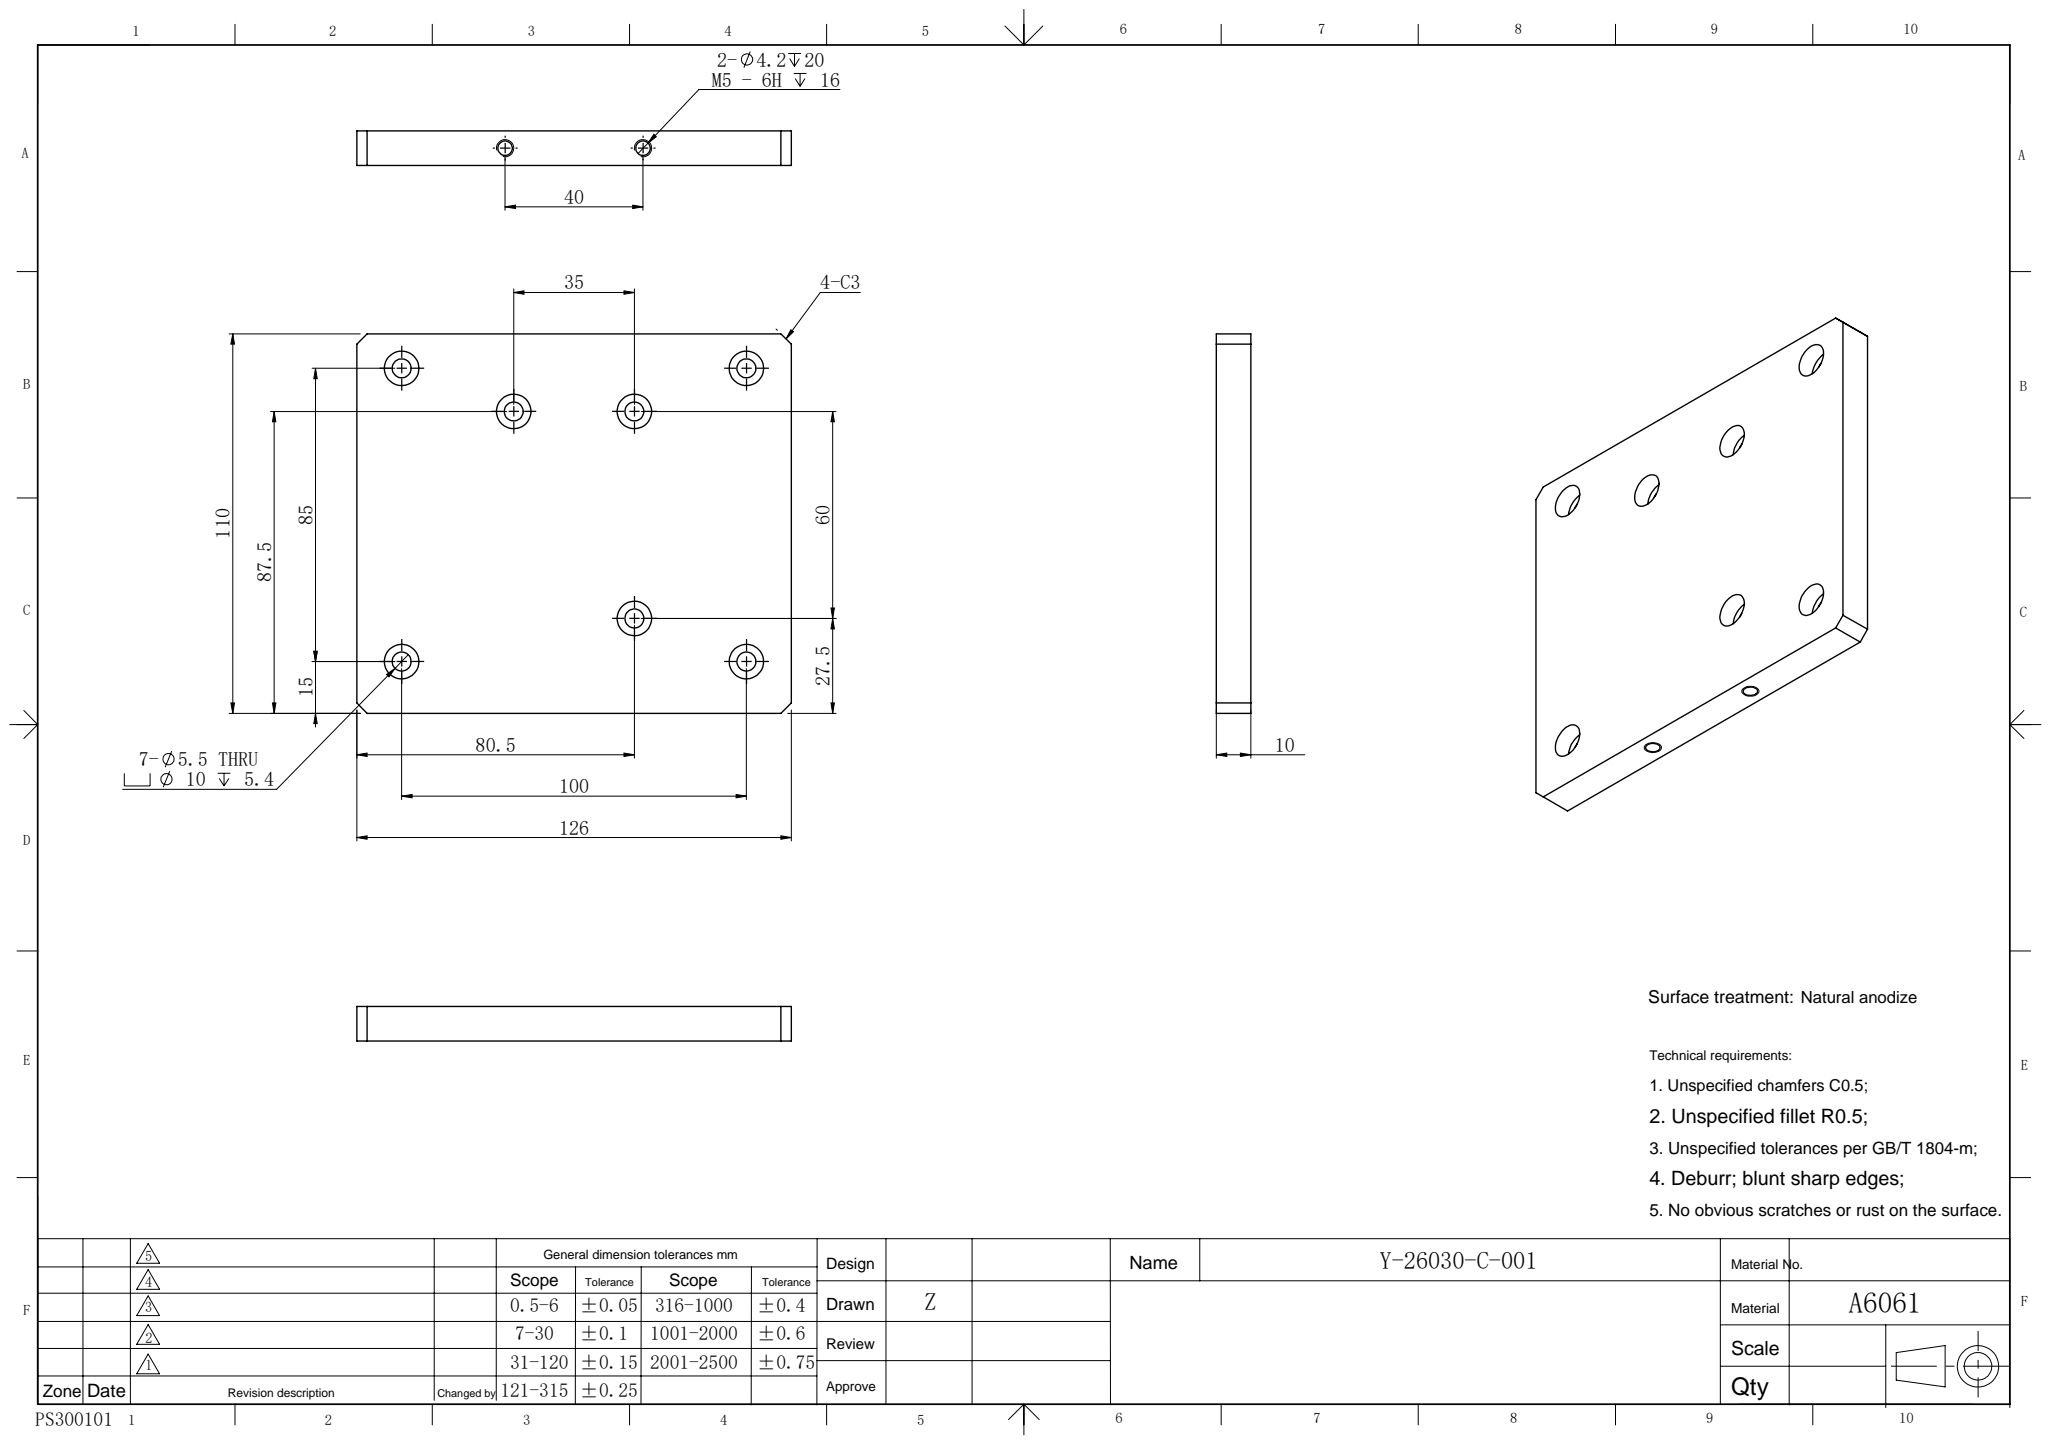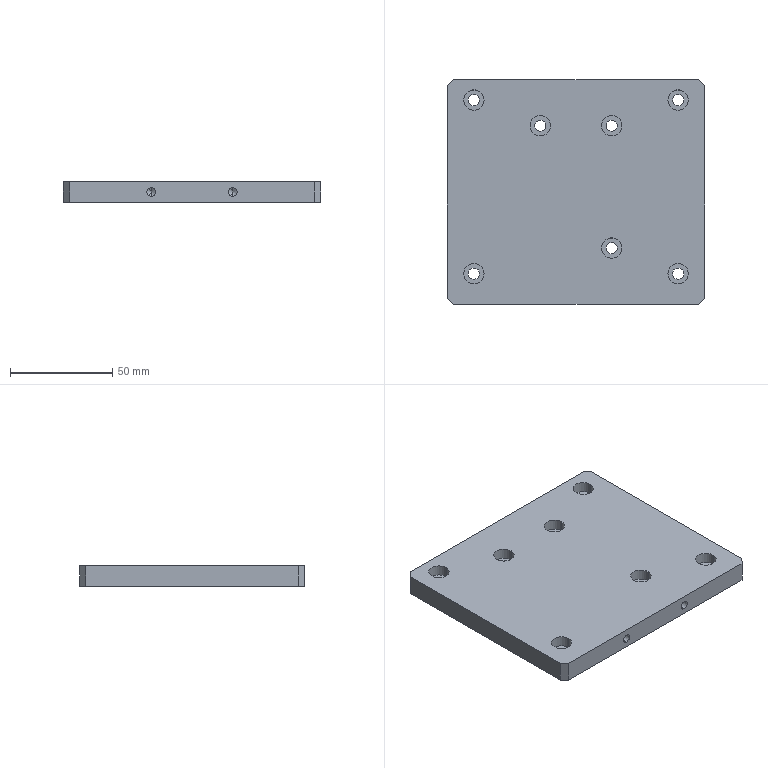Part | SolidWorks | features HoleWzd 2, Chamfer 1, Extrusion 1 | 1 solid | 53 faces | box 126 x 110 x 10 mm | volume 134120 mm3 | cylinder 32 | plane 17 | cone 4 | commonest cylinder face diameters 5.5 x14 10 x14 4.2 x4